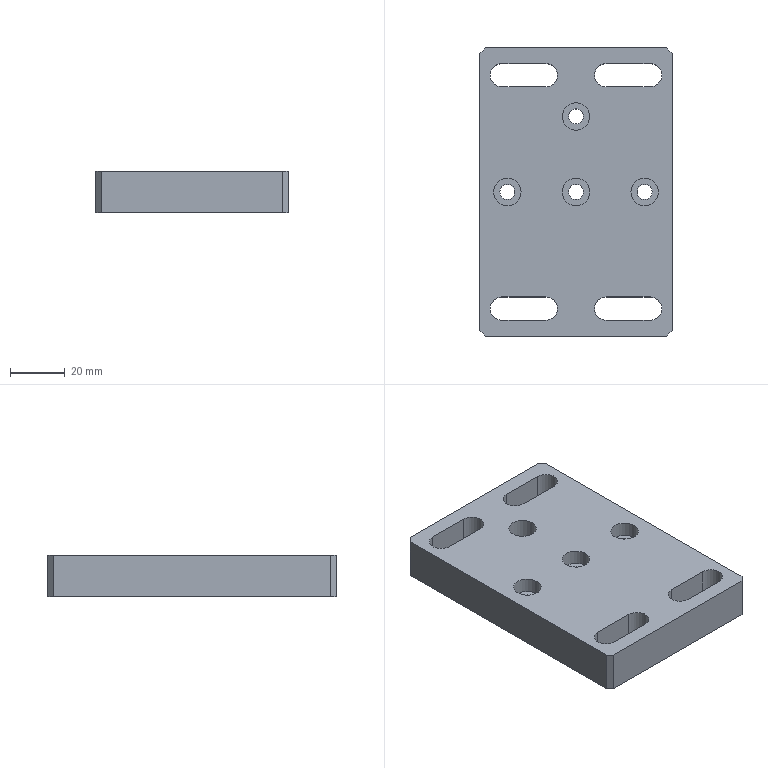CAM job | NX | 3-axis milling, drilling | part box 70 x 105 x 15 mm | stock box 75 x 110 x 20 mm
Tools:
number,name,description,diameter,corner_radius,flute_length,length,flutes
6,D6,平底铣刀-粗,6.0,0.0,25.0,75.0,2
9,D10,平底铣刀-粗,10.0,0.0,35.0,75.0,2
7,D6-J,平底铣刀-精,6.0,0.0,25.0,75.0,2
10,D10-J,平底铣刀-精,10.0,0.0,35.0,75.0,2
1,D80R0.8飞刀,圆鼻刀-粗,80.0,0.8,50.0,75.0,2
2,D6倒角刀,倒角刀,6.0,0.0,3.0,25.0,2
17,钻头5.5,Twist Drill 5 mm,5.5,0.0,52.0,54.0,2
Operations:
program,operation,operation_type,tool,method,geometry_group,spindle_rpm,surface_speed,feed_per_tooth,feed_cut,feed_plunge,cut_length_mm,path_length_mm,cut_time_min,machine_time_min
B,顶面_COPY,FaceMilling,D80R0.8飞刀,侧刃精光-切深K-步距G,W-B,5000.0,1256.637,0.1,1000.0,100.0,1990.0,3807.62,1.99,2.172
B,顶面_COPY_COPY,FaceMilling,D80R0.8飞刀,侧刃精光-切深K-步距G,W-B,5000.0,1256.637,0.1,1000.0,100.0,199.0,235.0,0.199,0.2026
B,平面去毛刺6X45L_COPY,SurfaceContour,D6倒角刀,爬面_倒角-切深0-步距G,W-B,6500.0,122.519,0.1154,1500.0,100.0,638.887,1115.947,0.4259,0.4736
A,顶面,FaceMilling,D80R0.8飞刀,侧刃精光-切深K-步距G,W-A,5000.0,1256.637,0.1,1000.0,100.0,199.0,235.0,0.199,0.2026
A,外形粗_2,VolumeBased25DMillingOperation,D10,METHOD,W-A,8000.0,251.327,0.3125,5000.0,80.0,7926.033,7979.833,1.585,1.591
A,沉头孔打点-深0.8,Operation,D6倒角刀,NONE,W-A,8000.0,150.796,0.0312,500.0,90.0,7.2,144.619,0.0144,0.0281
A,沉头孔-钻孔0段,Operation,钻头5.5,NONE,W-A,2000.0,34.557,0.0625,250.0,90.0,78.609,287.438,0.3144,0.3353
A,通腰槽粗_1,VolumeBased25DMillingOperation,D6,METHOD,W-A,6000.0,113.0,0.2083,2500.0,100.0,12715.278,13095.579,5.086,5.124
A,铣孔开粗D6_1,CylinderMilling,D6,NONE,W-A,8000.0,150.796,0.075,1200.0,100.0,197.135,243.635,0.1643,0.1689
A,铣孔开粗D6_2,CylinderMilling,D6,NONE,W-A,8000.0,150.796,0.075,1200.0,100.0,476.699,661.399,0.3972,0.4157
A,仅选体,SurfaceContour,D6倒角刀,METHOD,W-A,8000.0,150.796,0.1875,3000.0,100.0,601.344,980.037,0.2004,0.2383
A,铣倒角_1,PlanarMilling,D6倒角刀,NONE,W-A,8000.0,150.796,0.05,800.0,100.0,161.004,381.689,0.2013,0.2233
A,铣孔精光D6_1,CylinderMilling,D6-J,精光步距切深关,W-A,8000.0,150.796,0.0312,500.0,100.0,37.726,84.726,0.0755,0.0802
A,铣孔精光D6_2,CylinderMilling,D6-J,精光步距切深关,W-A,8000.0,150.796,0.0312,500.0,100.0,100.196,286.396,0.2004,0.219
A,腰槽精_1,VolumeBased25DMillingOperation,D6-J,METHOD,W-A,6000.0,113.0,0.0667,600.0,100.0,504.988,1047.656,0.8416,0.8959
A,外形半精_2,VolumeBased25DMillingOperation,D10-J,METHOD,W-A,8000.0,251.327,0.0625,1000.0,100.0,381.688,451.288,0.3817,0.3886